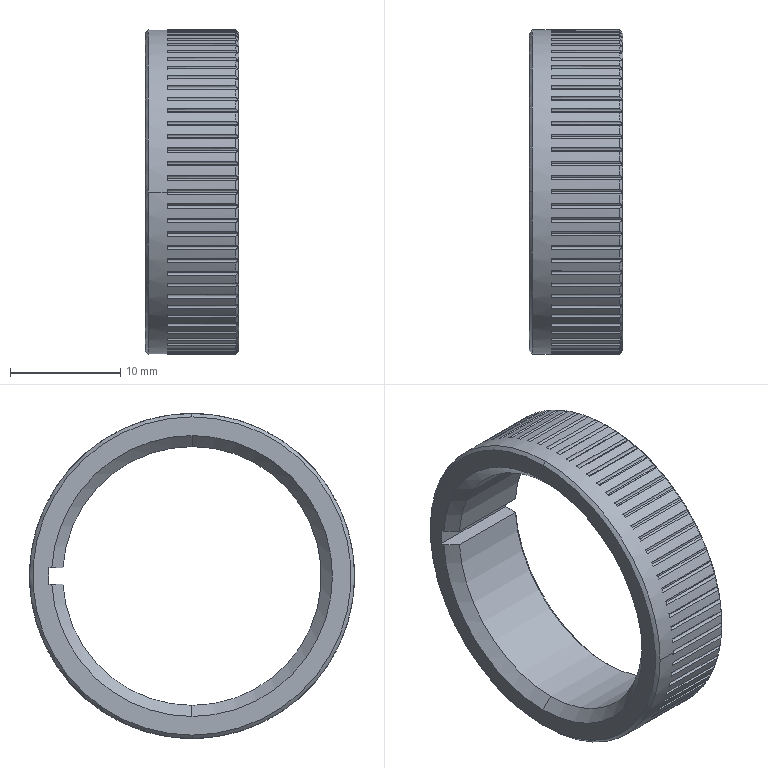Part | STEP file | handwheel.stp.STEP-270.STEP | 1 solid | 237 faces | box 8.5 x 29.5 x 29.5 mm | volume 2030 mm3 | cylinder 147 | plane 80 | cone 10 | commonest cylinder face diameters 0.4 x144 29.5 x2 23.5 x1